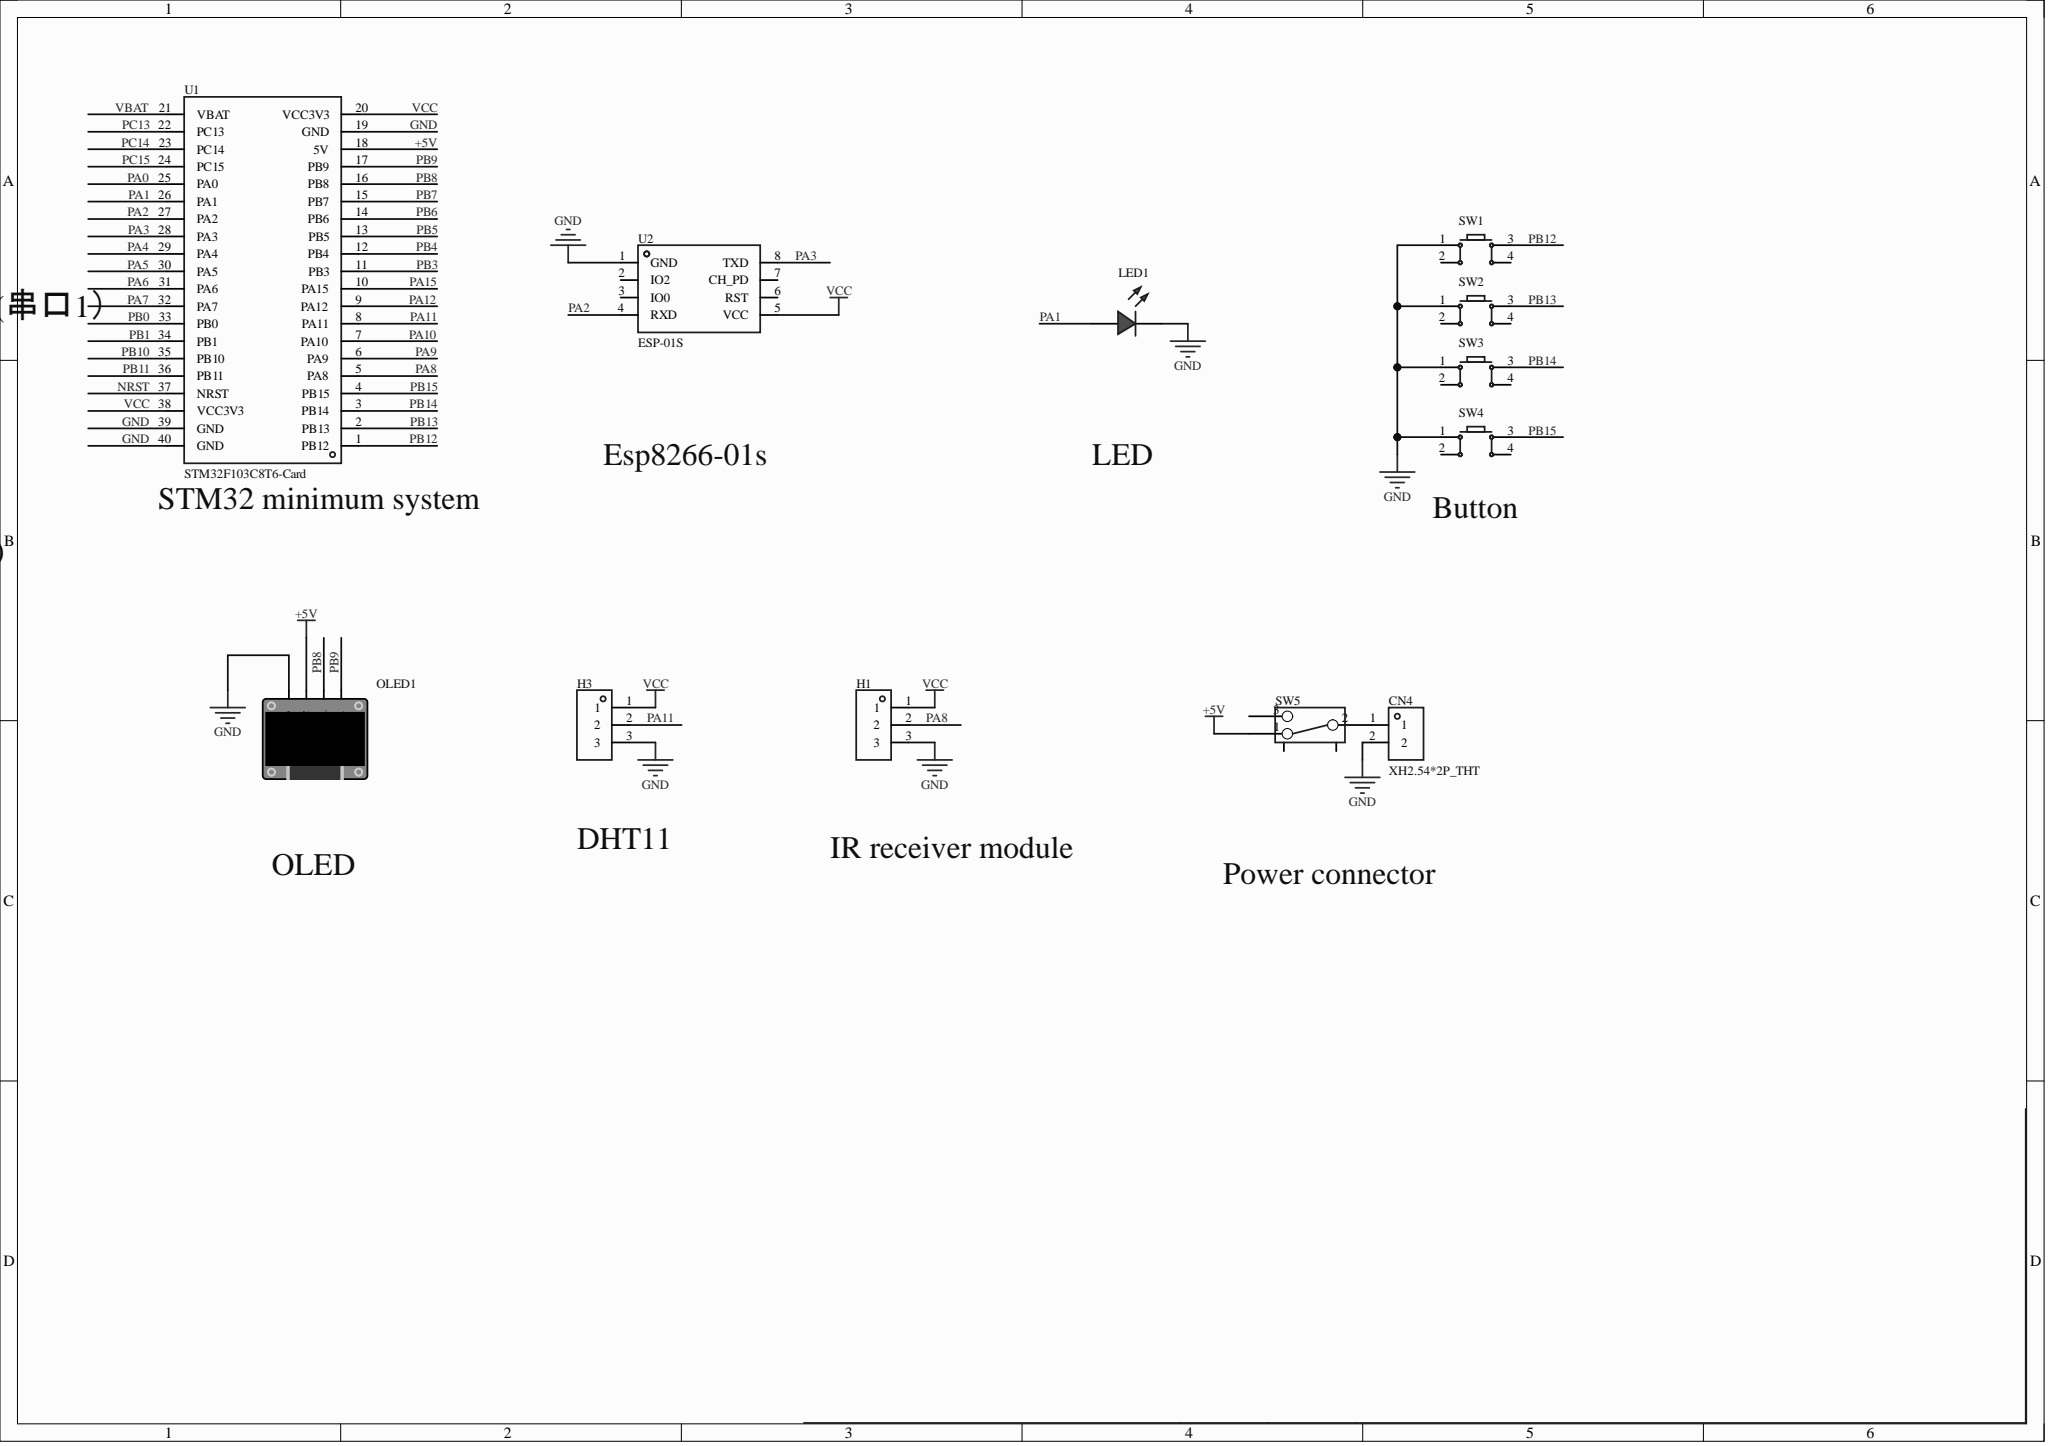Circuit board | Altium Designer | 12 parts | 15 nets
Bill of materials:
Comment,Description,Designator,Footprint,LibRef,Quantity
"XH2.54*2P_THT","","CN4","CONN-TH_2P-P2.50-XH2.54-2P","XH2.54*2P_直插","1"
"","","H1, H3","HDR-TH_3P-P2.54-V-F","HDR-F_2.54_1x3P","2"
"","","LED1","LED-TH_5mm","LED_TH-R_5mm","1"
"","","OLED1","0.96OLED_4P","0.96OLED模块_4P","1"
"","","SW1, SW2, SW3, SW4","SW-TH_4P-L6.0-W6.0-P4.50-LS6.5","Key_TH_6x6x6","4"
"","","SW5","拨动开关","拨动开关_正","1"
"STM32F103C8T6-Card","","U1","CONN-TH_L53.3-W22.9_STM32F103C8T6-CARD","STM32F103C8T6-Card","1"
"ESP-01S","","U2","WIFIM-TH_ESP-01S","ESP-01S_C111009","1"
Netlist (Protel format):
[
CN4
CONN-TH_2P-P2.50-XH2.54-2P
XH2.54*2P_THT



]
[
H1
HDR-TH_3P-P2.54-V-F




]
[
H3
HDR-TH_3P-P2.54-V-F




]
[
LED1
LED-TH_5mm




]
[
OLED1
0.96OLED_4P




]
[
SW1
SW-TH_4P-L6.0-W6.0-P4.50-LS6.5




]
[
SW2
SW-TH_4P-L6.0-W6.0-P4.50-LS6.5




]
[
SW3
SW-TH_4P-L6.0-W6.0-P4.50-LS6.5




]
[
SW4
SW-TH_4P-L6.0-W6.0-P4.50-LS6.5




]
[
SW5
拨动开关




]
[
U1
CONN-TH_L53.3-W22.9_STM32F103C8T6-CARD
STM32F103C8T6-Card



]
[
U2
WIFIM-TH_ESP-01S
ESP-01S



]
(
VCC
H1-1
H3-1
U1-20
U1-38
U2-5
)
(
PB15
SW4-3
U1-4
)
(
PB14
SW3-3
U1-3
)
(
PB13
SW2-3
U1-2
)
(
PB12
SW1-3
U1-1
)
(
PB9
OLED1-4
U1-17
)
(
PB8
OLED1-3
U1-16
)
(
PA11
H3-2
U1-8
)
(
PA8
H1-2
U1-5
)
(
PA3
U1-28
U2-8
)
(
PA2
U1-27
U2-4
)
(
PA1
LED1-1
U1-26
)
(
NetCN4_1
CN4-1
SW5-2
)
(
GND
CN4-2
H1-3
H3-3
LED1-2
OLED1-1
SW1-1
SW2-1
SW3-1
SW4-1
U1-19
U1-39
U1-40
U2-1
)
(
+5V
OLED1-2
SW5-1
U1-18
)